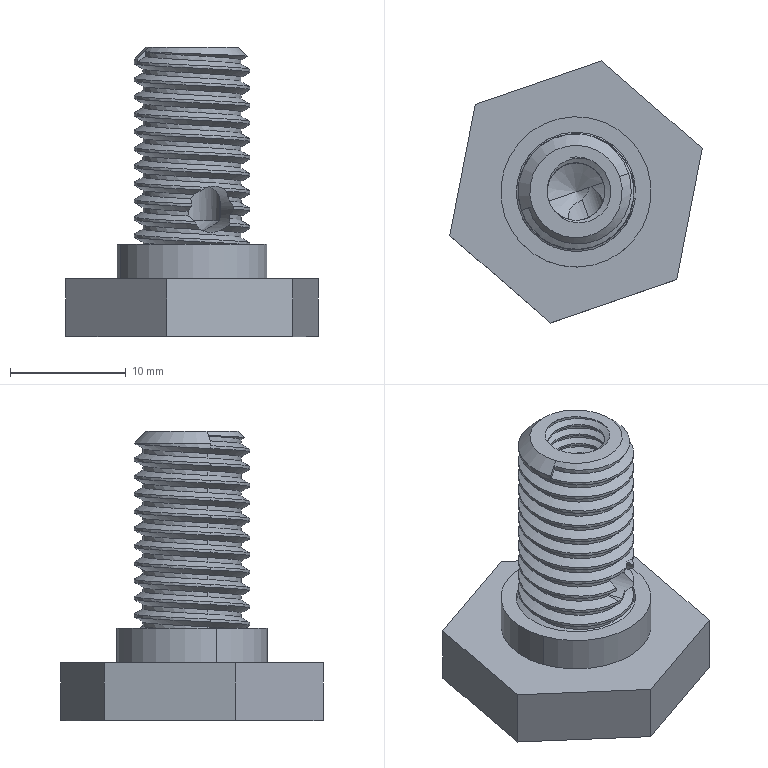Part | SolidWorks | features BaseBody 1 | 1 solid | 126 faces | box 21.836 x 22.67 x 25 mm | volume 2862 mm3 | cylinder 97 | plane 14 | spline 10 | cone 5 | commonest cylinder face diameters 10 x26 8.5 x25 5 x21 6 x21 4 x2 13 x2